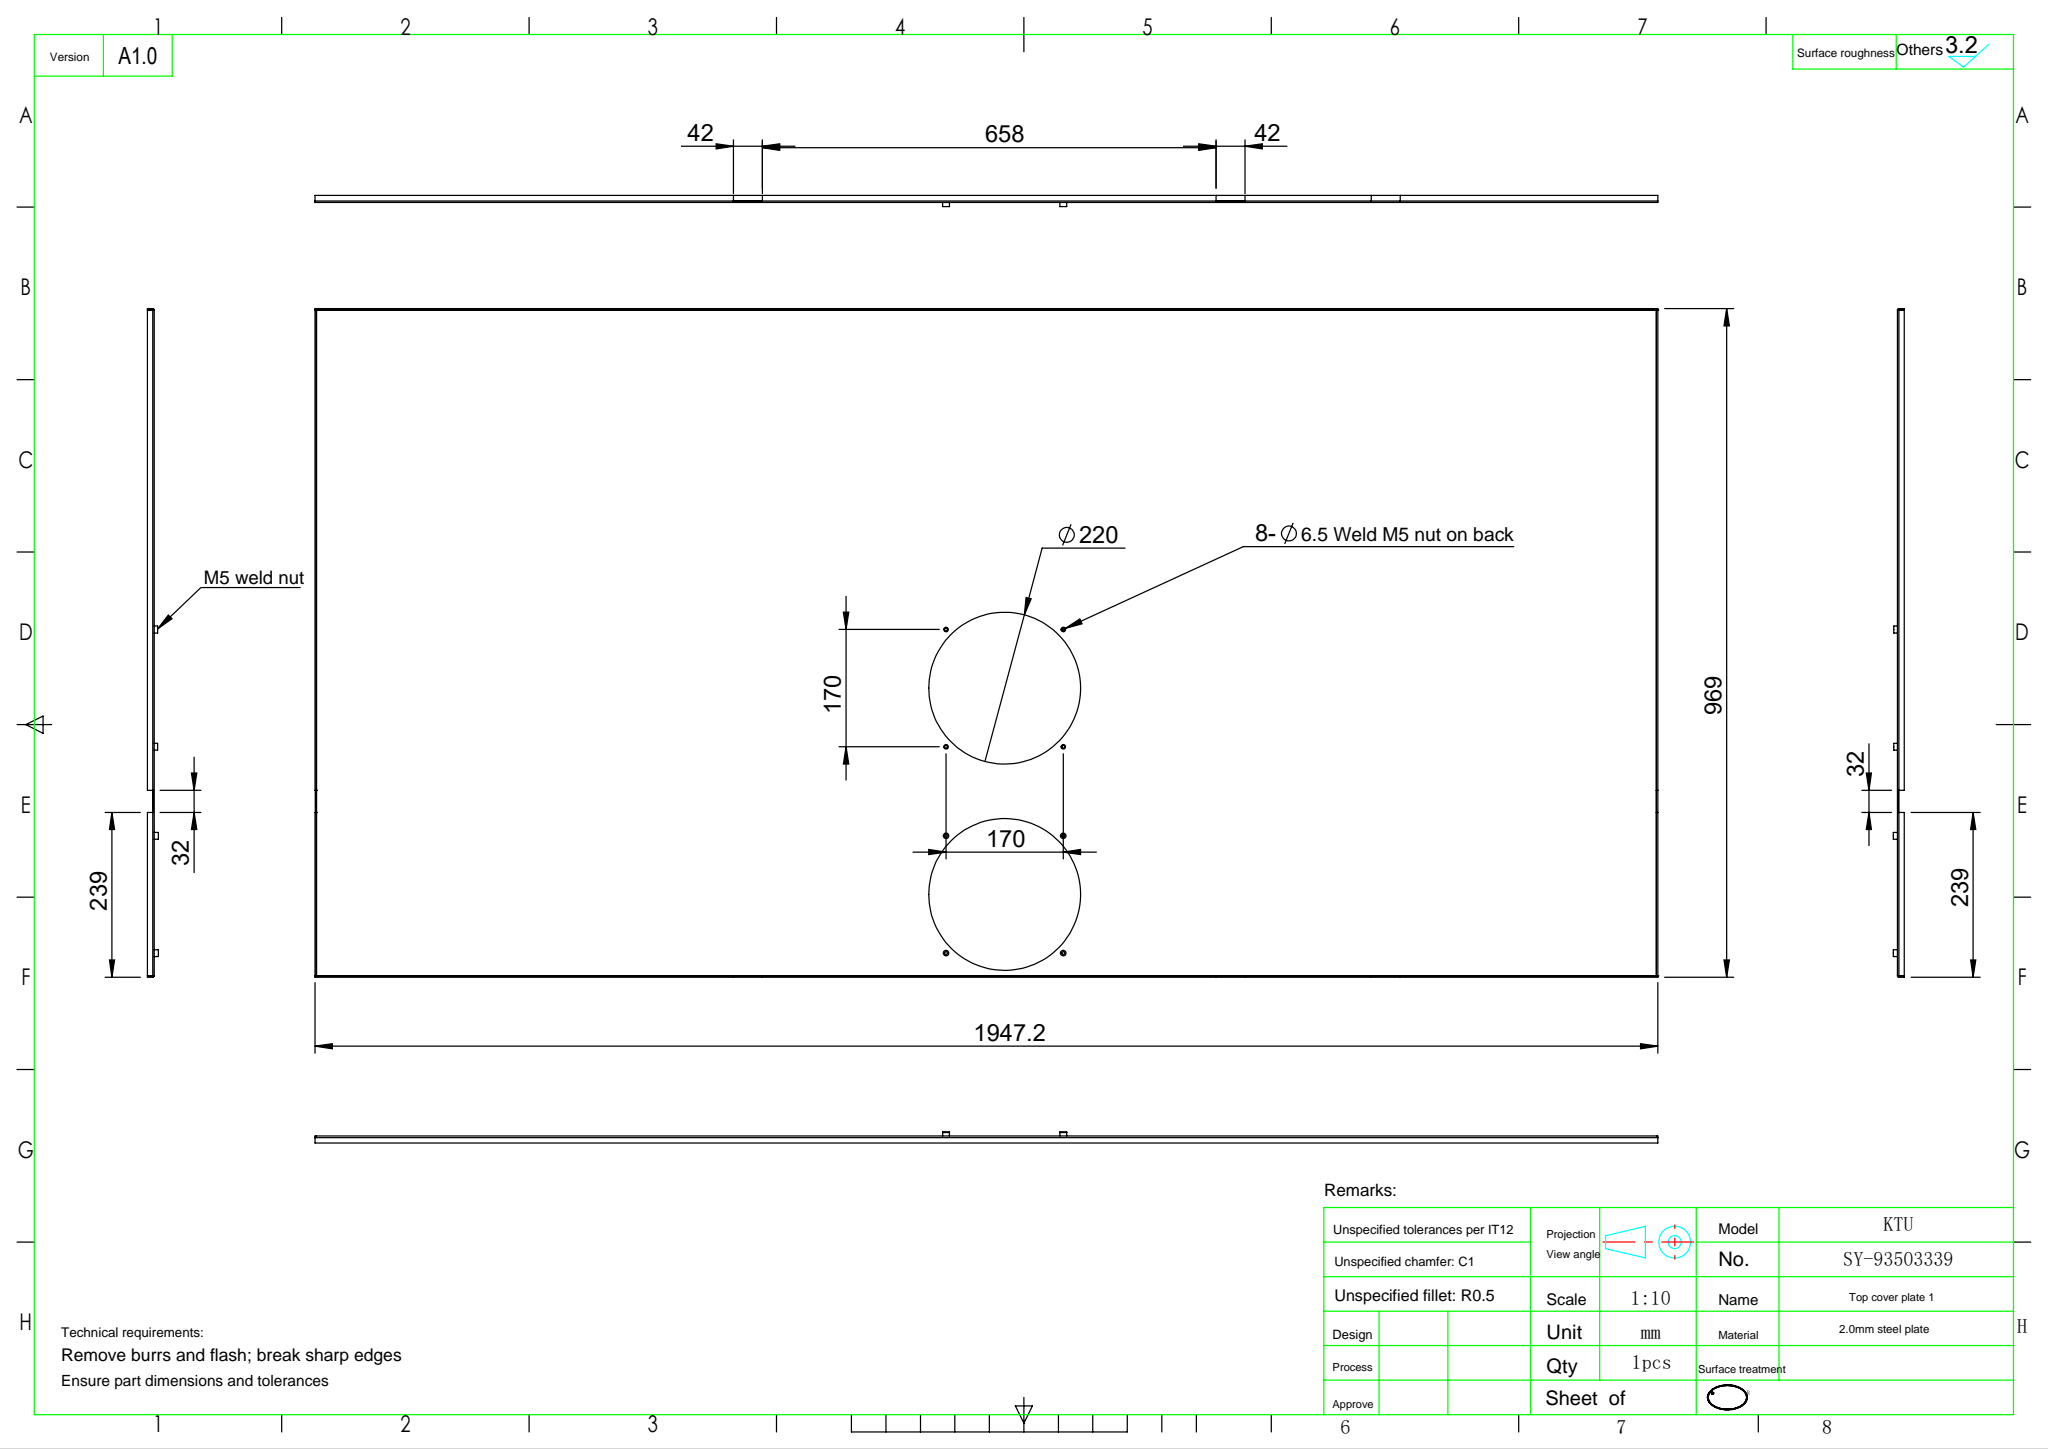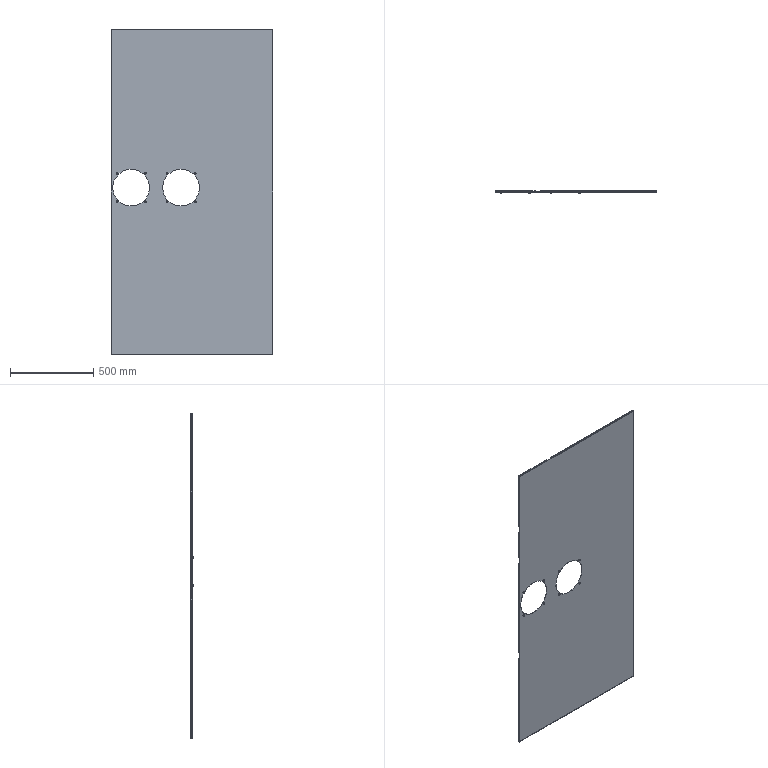Part | SolidWorks | features Cut 5, ICE 4, EdgeFlange 1, FlatPattern 1, MirrorPattern 1, SMBaseFlange 1, SheetMetal 1 | 5 solids | 148 faces | box 969 x 16 x 1947 mm | volume 3707899 mm3 | plane 88 | cylinder 60 | commonest cylinder face diameters 4.2 x16 10 x16 6.5 x8 8 x8 0.4 x4 4.4 x4